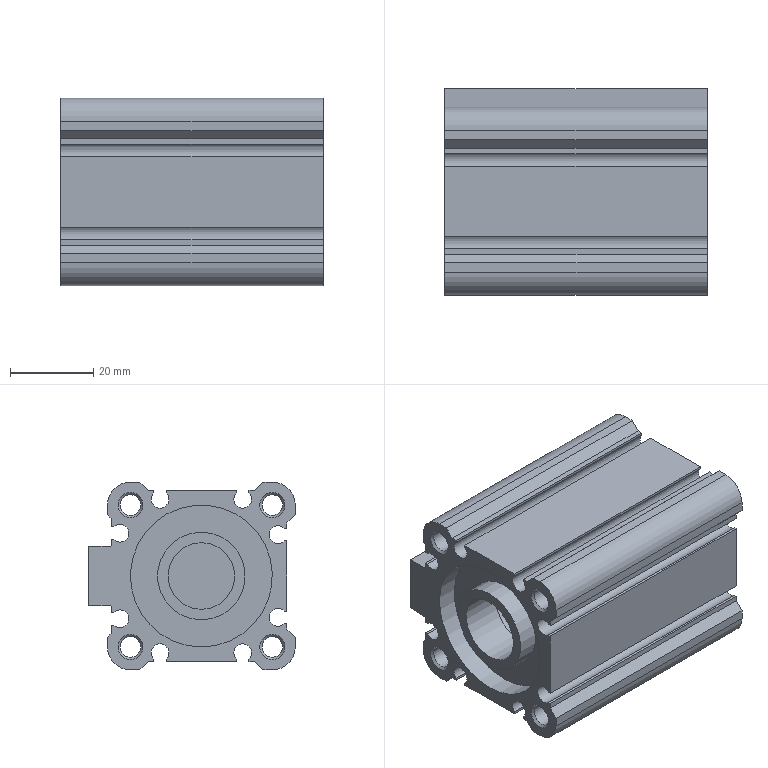Part | NX | 1 solid | 106 faces | box 63 x 49.5 x 45 mm | volume 69436 mm3 | plane 65 | cylinder 31 | cone 10 | commonest cylinder face diameters 4.26 x8 4.917 x8 6 x4 11 x4 8.566 x2 34 x2